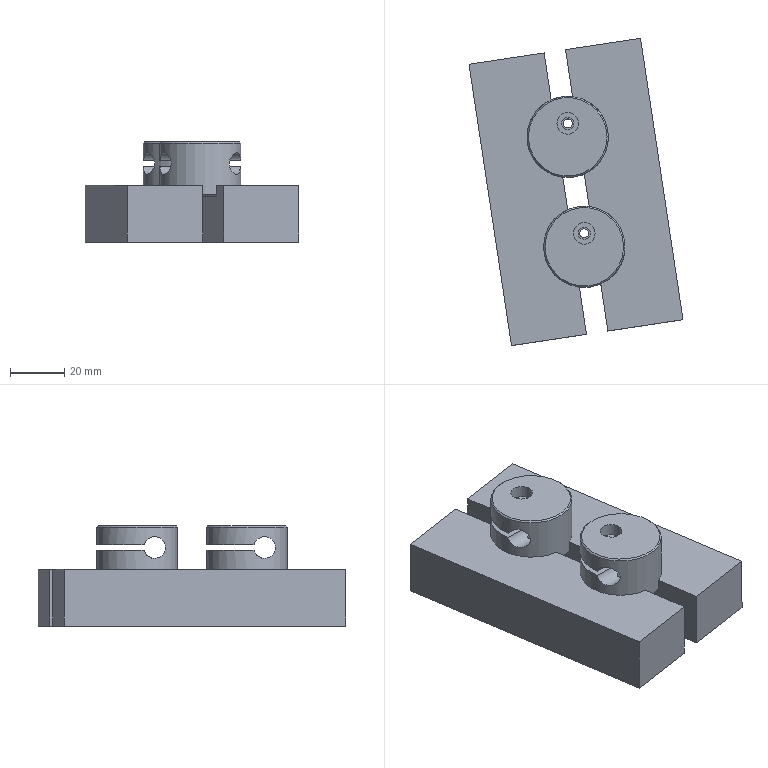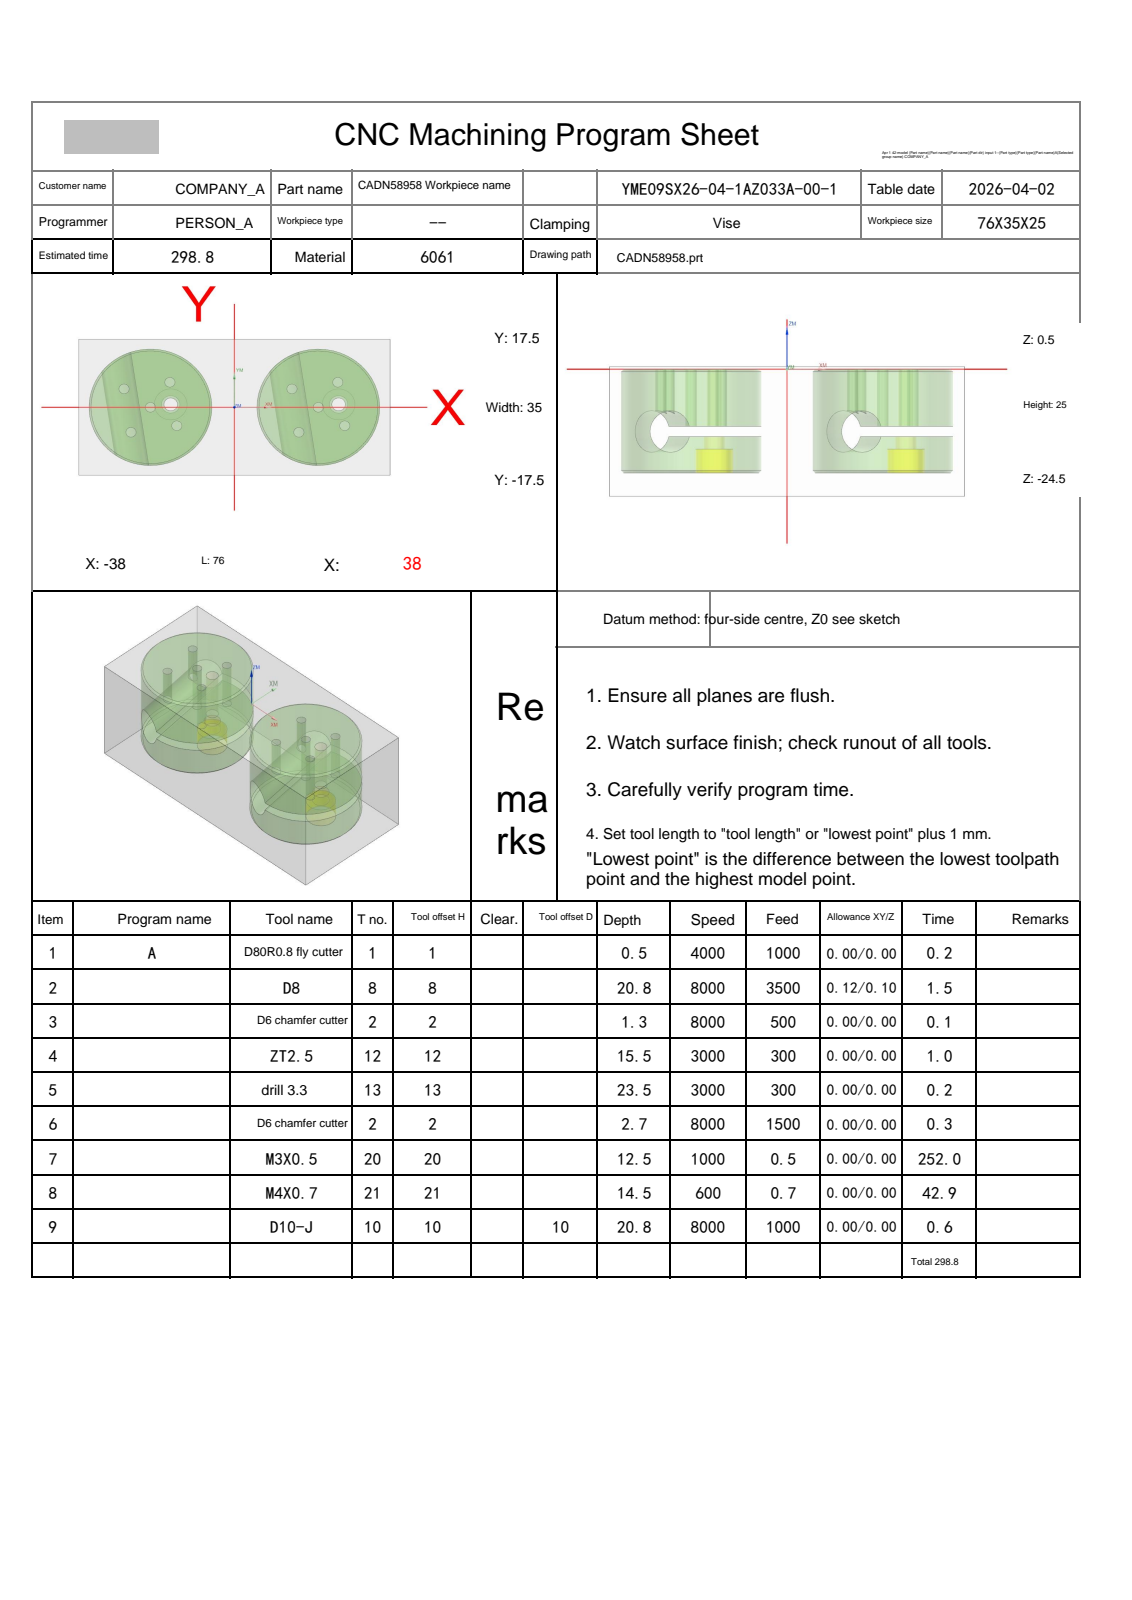NC program | NX | posted by the shop | part box 78.946 x 113.372 x 37 mm
Lines 1 to 34 of 2409:
%
O0001
(Machine time: 572.41 MIN)
(===Total Tool:8===)
(T1=D80R0.8 fly cutter D=80.  R=0.8  D-  H01 Z=0.    )
(T8=D8      D=8.   R=0.   D-  H08 Z=-20.3 )
(T2=D6 chamfer cutter   D=6.   R=0.   D-  H02 Z=-2.2  )
(T12=ZT2.5  D=2.5  DR_a=118 D-  H12 Z=-15.  )
(T13=drill 3.3  D=3.3  DR_a=118 D-  H13 Z=-23.  )
(T20=M3X0.5 D=2.5  DR_a=180 D-  H20 Z=-12.  )
(T21=M4X0.7 D=3.3  DR_a=180 D-  H21 Z=-14.  )
(T10=D10-J  D=10.  R=0.   D10 H10 Z=-20.3 )
G80 G90 G17 G49 G40
G91 G28 Z0
M01
N1 T01 M06
(D80R0.8 fly cutter  D=80. R=0.8 H=01 ce=0.00 di=0.00)
G00 G90 G54 X-80.5 Y0.0 M03 S4000
G43 H01 Z20.
M08
Z2.
G01 Z0.0 F1000.
X-75.5
X75.5
X80.5
Z2.
G00 Z20.
G91 G28 Z0.0
M05
M09
G91 G28 Z0.0
M01